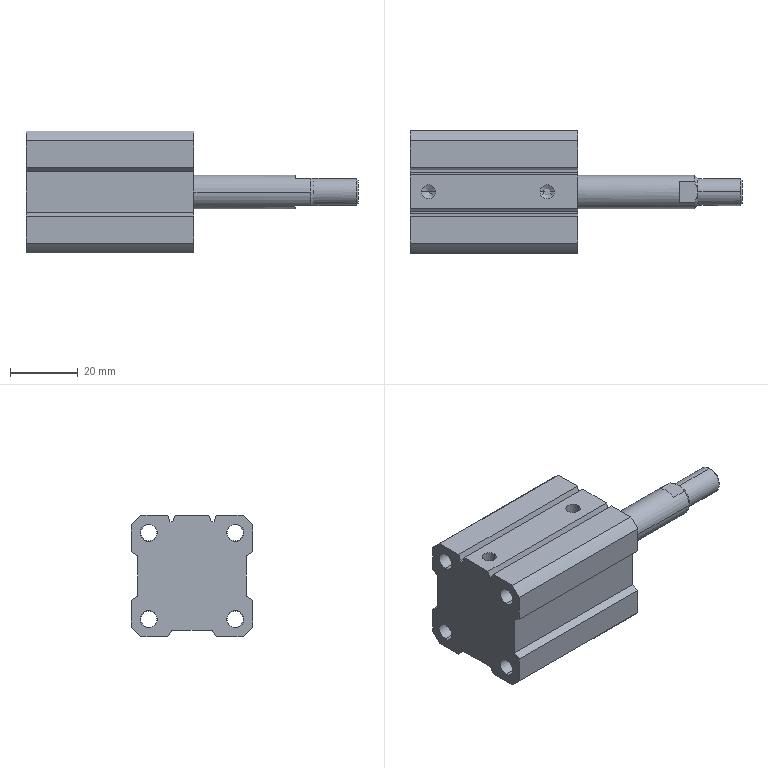Part | STEP file | Cylinder CDQ2A-20×30-DM Extend | 2 solids | 92 faces | box 98 x 36 x 36 mm | volume 59217 mm3 | cylinder 36 | plane 32 | cone 24 | commonest cylinder face diameters 5 x16 4.8 x8 4.2 x4 47 x4 8 x2 10 x2